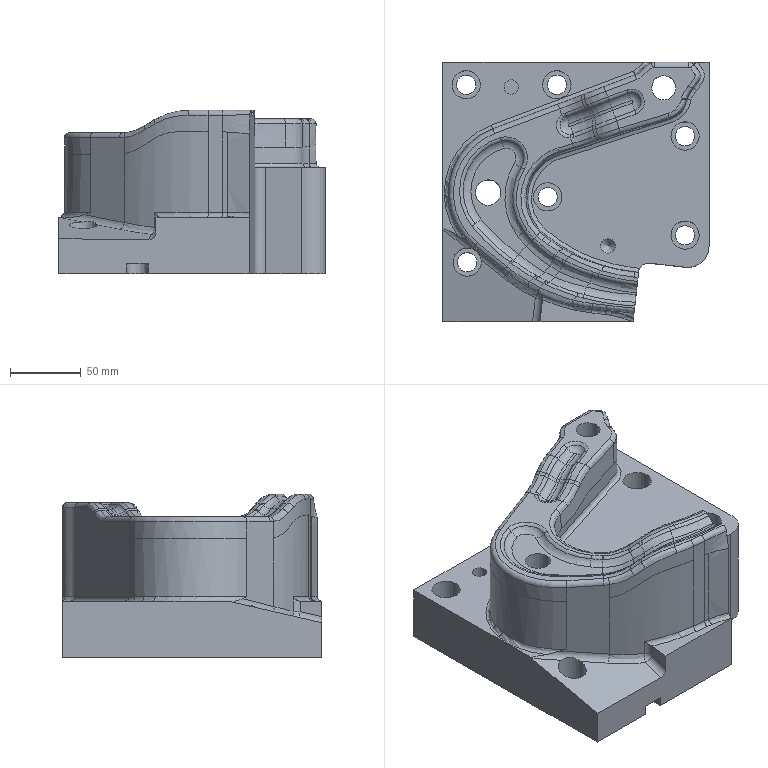Part | NX | features 23 2 | 1 solid | 219 faces | box 188 x 183.095 x 115.4 mm | volume 2254914 mm3 | spline 77 | cylinder 62 | plane 48 | torus 30 | sphere 1 | cone 1 | commonest cylinder face diameters 7 x8 6 x6 13.5 x6 20 x6 10 x5 13 x4